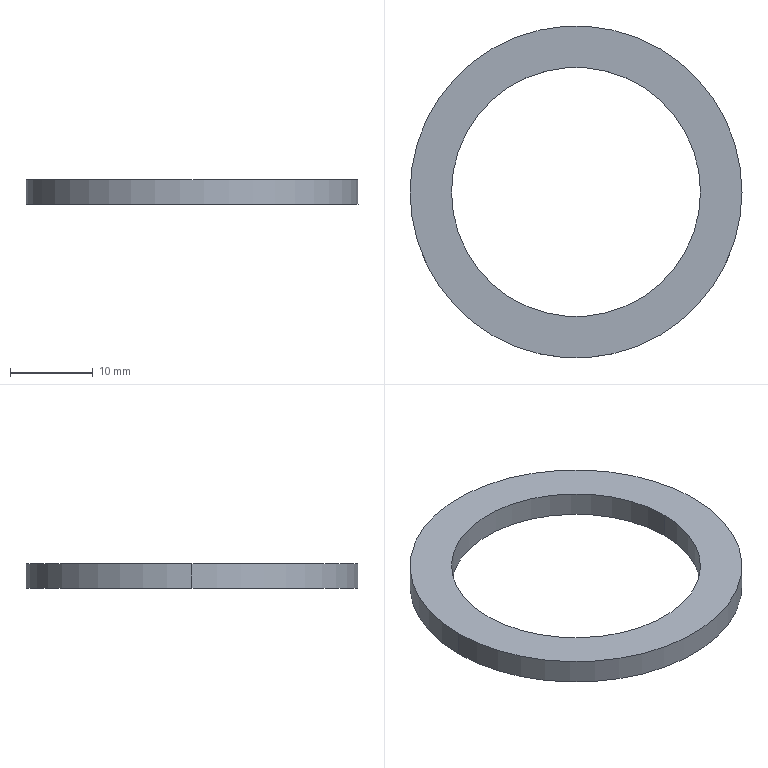Part | SolidWorks | features BaseBody 1 | 1 solid | 6 faces | box 40 x 40 x 3 mm | volume 1649 mm3 | cylinder 4 | plane 2 | commonest cylinder face diameters 30 x2 40 x2
STEP:
#1=CARTESIAN_POINT('',(-15.,0.,1.5));
#2=VERTEX_POINT('',#1);
#3=CARTESIAN_POINT('',(15.,0.,1.5));
#4=VERTEX_POINT('',#3);
#5=CARTESIAN_POINT('',(0.,0.,1.5));
#6=DIRECTION('',(0.,0.,1.));
#7=DIRECTION('',(1.,0.,0.));
#8=AXIS2_PLACEMENT_3D('',#5,#6,#7);
#9=CIRCLE('',#8,15.);
#10=EDGE_CURVE('',#2,#4,#9,.T.);
#11=ORIENTED_EDGE('',*,*,#10,.T.);
#12=CARTESIAN_POINT('',(15.,0.,-1.5));
#13=VERTEX_POINT('',#12);
#14=CARTESIAN_POINT('',(15.,0.,1.5));
#15=DIRECTION('',(0.,0.,-1.));
#16=VECTOR('',#15,1000.);
#17=LINE('',#14,#16);
#18=EDGE_CURVE('',#4,#13,#17,.T.);
#19=ORIENTED_EDGE('',*,*,#18,.T.);
#20=CARTESIAN_POINT('',(-15.,0.,-1.5));
#21=VERTEX_POINT('',#20);
#22=CARTESIAN_POINT('',(0.,0.,-1.5));
#23=DIRECTION('',(0.,0.,1.));
#24=DIRECTION('',(1.,0.,0.));
#25=AXIS2_PLACEMENT_3D('',#22,#23,#24);
#26=CIRCLE('',#25,15.);
#27=EDGE_CURVE('',#21,#13,#26,.T.);
#28=ORIENTED_EDGE('',*,*,#27,.F.);
#29=CARTESIAN_POINT('',(-15.,0.,1.5));
#30=DIRECTION('',(0.,0.,-1.));
#31=VECTOR('',#30,1000.);
#32=LINE('',#29,#31);
#33=EDGE_CURVE('',#2,#21,#32,.T.);
#34=ORIENTED_EDGE('',*,*,#33,.F.);
#35=EDGE_LOOP('',(#11,#19,#28,#34));
#36=FACE_OUTER_BOUND('',#35,.T.);
#37=CARTESIAN_POINT('',(0.,0.,1.5));
#38=DIRECTION('',(0.,0.,-1.));
#39=DIRECTION('',(-1.,0.,0.));
#40=AXIS2_PLACEMENT_3D('',#37,#38,#39);
#41=CYLINDRICAL_SURFACE('',#40,15.);
#42=ADVANCED_FACE('',(#36),#41,.F.);
#43=CARTESIAN_POINT('',(20.,0.,1.5));
#44=VERTEX_POINT('',#43);
#45=CARTESIAN_POINT('',(-20.,0.,1.5));
#46=VERTEX_POINT('',#45);
#47=CARTESIAN_POINT('',(0.,0.,1.5));
#48=DIRECTION('',(0.,0.,1.));
#49=DIRECTION('',(1.,0.,0.));
#50=AXIS2_PLACEMENT_3D('',#47,#48,#49);
#51=CIRCLE('',#50,20.);
#52=EDGE_CURVE('',#44,#46,#51,.T.);
#53=ORIENTED_EDGE('',*,*,#52,.F.);
#54=CARTESIAN_POINT('',(20.,0.,-1.5));
#55=VERTEX_POINT('',#54);
#56=CARTESIAN_POINT('',(20.,0.,1.5));
#57=DIRECTION('',(0.,0.,-1.));
#58=VECTOR('',#57,1000.);
#59=LINE('',#56,#58);
#60=EDGE_CURVE('',#44,#55,#59,.T.);
#61=ORIENTED_EDGE('',*,*,#60,.T.);
#62=CARTESIAN_POINT('',(-20.,0.,-1.5));
#63=VERTEX_POINT('',#62);
#64=CARTESIAN_POINT('',(0.,0.,-1.5));
#65=DIRECTION('',(0.,0.,1.));
#66=DIRECTION('',(1.,0.,0.));
#67=AXIS2_PLACEMENT_3D('',#64,#65,#66);
#68=CIRCLE('',#67,20.);
#69=EDGE_CURVE('',#55,#63,#68,.T.);
#70=ORIENTED_EDGE('',*,*,#69,.T.);
#71=CARTESIAN_POINT('',(-20.,0.,1.5));
#72=DIRECTION('',(0.,0.,-1.));
#73=VECTOR('',#72,1000.);
#74=LINE('',#71,#73);
#75=EDGE_CURVE('',#46,#63,#74,.T.);
#76=ORIENTED_EDGE('',*,*,#75,.F.);
#77=EDGE_LOOP('',(#53,#61,#70,#76));
#78=FACE_OUTER_BOUND('',#77,.T.);
#79=CARTESIAN_POINT('',(0.,0.,1.5));
#80=DIRECTION('',(0.,0.,-1.));
#81=DIRECTION('',(-1.,0.,0.));
#82=AXIS2_PLACEMENT_3D('',#79,#80,#81);
#83=CYLINDRICAL_SURFACE('',#82,20.);
#84=ADVANCED_FACE('',(#78),#83,.T.);
#85=ORIENTED_EDGE('',*,*,#27,.T.);
#86=CARTESIAN_POINT('',(0.,0.,-1.5));
#87=DIRECTION('',(0.,0.,1.));
#88=DIRECTION('',(1.,0.,0.));
#89=AXIS2_PLACEMENT_3D('',#86,#87,#88);
#90=CIRCLE('',#89,15.);
#91=EDGE_CURVE('',#13,#21,#90,.T.);
#92=ORIENTED_EDGE('',*,*,#91,.T.);
#93=EDGE_LOOP('',(#85,#92));
#94=FACE_BOUND('',#93,.T.);
#95=CARTESIAN_POINT('',(0.,0.,-1.5));
#96=DIRECTION('',(0.,0.,1.));
#97=DIRECTION('',(1.,0.,0.));
#98=AXIS2_PLACEMENT_3D('',#95,#96,#97);
#99=CIRCLE('',#98,20.);
#100=EDGE_CURVE('',#63,#55,#99,.T.);
#101=ORIENTED_EDGE('',*,*,#100,.F.);
#102=ORIENTED_EDGE('',*,*,#69,.F.);
#103=EDGE_LOOP('',(#101,#102));
#104=FACE_OUTER_BOUND('',#103,.T.);
#105=CARTESIAN_POINT('',(0.,0.,-1.5));
#106=DIRECTION('',(0.,0.,1.));
#107=DIRECTION('',(1.,0.,0.));
#108=AXIS2_PLACEMENT_3D('',#105,#106,#107);
#109=PLANE('',#108);
#110=ADVANCED_FACE('',(#94,#104),#109,.F.);
#111=ORIENTED_EDGE('',*,*,#10,.F.);
#112=CARTESIAN_POINT('',(0.,0.,1.5));
#113=DIRECTION('',(0.,0.,1.));
#114=DIRECTION('',(1.,0.,0.));
#115=AXIS2_PLACEMENT_3D('',#112,#113,#114);
#116=CIRCLE('',#115,15.);
#117=EDGE_CURVE('',#4,#2,#116,.T.);
#118=ORIENTED_EDGE('',*,*,#117,.F.);
#119=EDGE_LOOP('',(#111,#118));
#120=FACE_BOUND('',#119,.T.);
#121=CARTESIAN_POINT('',(0.,0.,1.5));
#122=DIRECTION('',(0.,0.,1.));
#123=DIRECTION('',(1.,0.,0.));
#124=AXIS2_PLACEMENT_3D('',#121,#122,#123);
#125=CIRCLE('',#124,20.);
#126=EDGE_CURVE('',#46,#44,#125,.T.);
#127=ORIENTED_EDGE('',*,*,#126,.T.);
#128=ORIENTED_EDGE('',*,*,#52,.T.);
#129=EDGE_LOOP('',(#127,#128));
#130=FACE_OUTER_BOUND('',#129,.T.);
#131=CARTESIAN_POINT('',(0.,0.,1.5));
#132=DIRECTION('',(0.,0.,1.));
#133=DIRECTION('',(1.,0.,0.));
#134=AXIS2_PLACEMENT_3D('',#131,#132,#133);
#135=PLANE('',#134);
#136=ADVANCED_FACE('',(#120,#130),#135,.T.);
#137=ORIENTED_EDGE('',*,*,#60,.F.);
#138=ORIENTED_EDGE('',*,*,#126,.F.);
#139=ORIENTED_EDGE('',*,*,#75,.T.);
#140=ORIENTED_EDGE('',*,*,#100,.T.);
#141=EDGE_LOOP('',(#137,#138,#139,#140));
#142=FACE_OUTER_BOUND('',#141,.T.);
#143=CARTESIAN_POINT('',(0.,0.,1.5));
#144=DIRECTION('',(0.,0.,-1.));
#145=DIRECTION('',(-1.,0.,0.));
#146=AXIS2_PLACEMENT_3D('',#143,#144,#145);
#147=CYLINDRICAL_SURFACE('',#146,20.);
#148=ADVANCED_FACE('',(#142),#147,.T.);
#149=ORIENTED_EDGE('',*,*,#18,.F.);
#150=ORIENTED_EDGE('',*,*,#117,.T.);
#151=ORIENTED_EDGE('',*,*,#33,.T.);
#152=ORIENTED_EDGE('',*,*,#91,.F.);
#153=EDGE_LOOP('',(#149,#150,#151,#152));
#154=FACE_OUTER_BOUND('',#153,.T.);
#155=CARTESIAN_POINT('',(0.,0.,1.5));
#156=DIRECTION('',(0.,0.,-1.));
#157=DIRECTION('',(-1.,0.,0.));
#158=AXIS2_PLACEMENT_3D('',#155,#156,#157);
#159=CYLINDRICAL_SURFACE('',#158,15.);
#160=ADVANCED_FACE('',(#154),#159,.F.);
#161=CLOSED_SHELL('',(#42,#84,#110,#136,#148,#160));
#162=MANIFOLD_SOLID_BREP('',#161);
#163=CARTESIAN_POINT('',(0.,0.,0.));
#164=DIRECTION('',(0.,0.,1.));
#165=DIRECTION('',(1.,0.,0.));
#166=AXIS2_PLACEMENT_3D('',#163,#164,#165);
#167=(LENGTH_UNIT()NAMED_UNIT(*)SI_UNIT(.MILLI.,.METRE.));
#168=UNCERTAINTY_MEASURE_WITH_UNIT(LENGTH_MEASURE(0.00001),#167,'','');
#169=(NAMED_UNIT(*)PLANE_ANGLE_UNIT()SI_UNIT($,.RADIAN.));
#170=(NAMED_UNIT(*)SI_UNIT($,.STERADIAN.)SOLID_ANGLE_UNIT());
#171=(GEOMETRIC_REPRESENTATION_CONTEXT(3)GLOBAL_UNCERTAINTY_ASSIGNED_CONTEXT((#168))GLOBAL_UNIT_ASSIGNED_CONTEXT((#167,#169,#170))REPRESENTATION_CONTEXT('',''));
#172=ADVANCED_BREP_SHAPE_REPRESENTATION('',(#162,#166),#171);